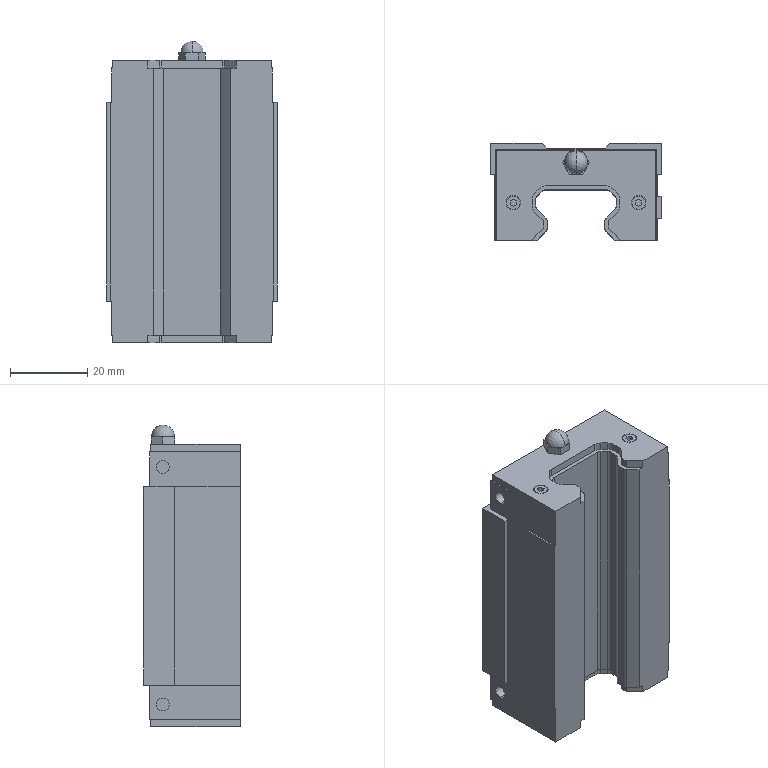Part | SolidWorks | features ICE 10, MirrorPattern 3, Chamfer 1, Extrusion 1, HoleWzd 1, Revolution 1 | 1 solid | 202 faces | box 44 x 25 x 77.9 mm | volume 57159 mm3 | plane 122 | cylinder 62 | cone 16 | sphere 2 | commonest cylinder face diameters 4.4 x12 2.4 x10 0.4 x8 3.3 x8 3.45 x8 3.75 x8